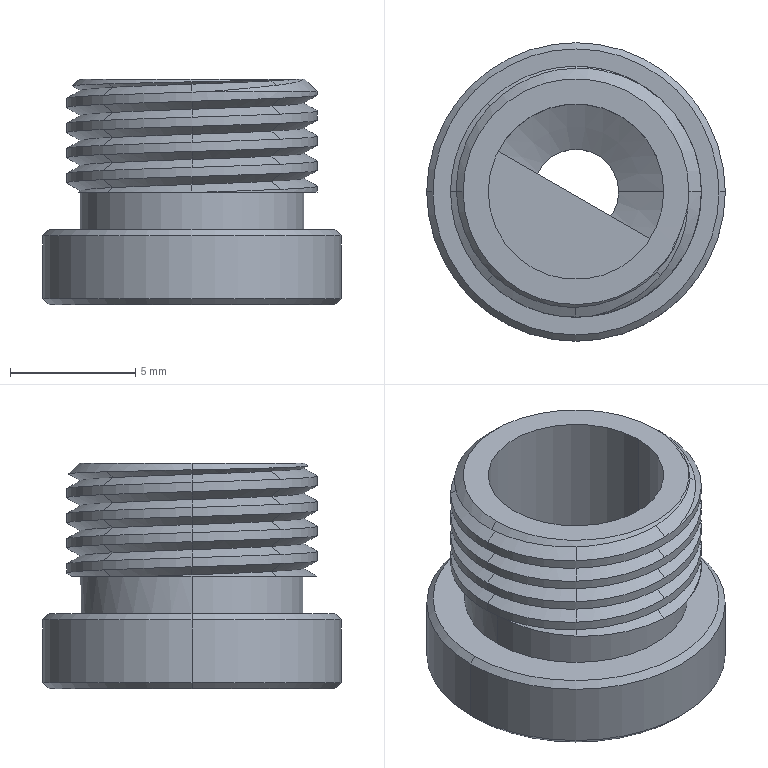Part | NX | features BREP 1 | 1 solid | 117 faces | box 11.9 x 11.9 x 9 mm | volume 484.643 mm3 | spline 76 | cylinder 22 | cone 15 | plane 4 | commonest cylinder face diameters 10 x10 1.5 x4 3.4 x2 7 x2 8.9 x2 11.9 x2